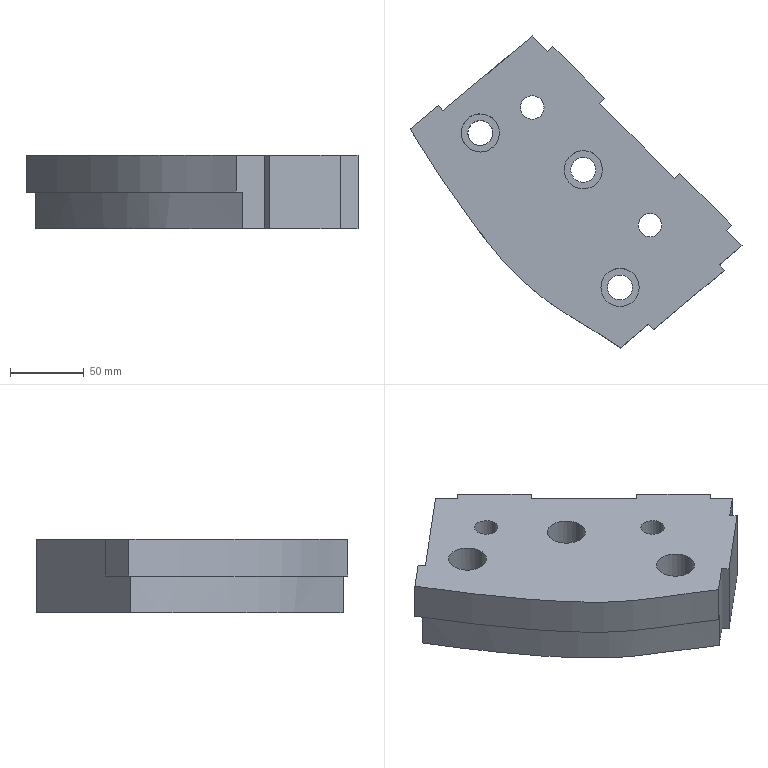Part | NX | features solid 2 | 1 solid | 33 faces | box 225.745 x 212.12 x 50 mm | volume 1112027 mm3 | plane 23 | cylinder 8 | spline 2 | commonest cylinder face diameters 17 x3 26 x3 16 x2
STEP:
#1=CARTESIAN_POINT('',(142.732,-499.403,0.));
#2=VERTEX_POINT('',#1);
#3=CARTESIAN_POINT('',(158.053,-486.547,0.));
#4=VERTEX_POINT('',#3);
#5=CARTESIAN_POINT('',(75.334,-555.957,0.));
#6=DIRECTION('',(0.766,0.6428,0.));
#7=VECTOR('',#6,1000.);
#8=LINE('',#5,#7);
#9=EDGE_CURVE('',#2,#4,#8,.T.);
#10=ORIENTED_EDGE('',*,*,#9,.F.);
#11=CARTESIAN_POINT('',(142.732,-499.403,-50.));
#12=VERTEX_POINT('',#11);
#13=CARTESIAN_POINT('',(142.732,-499.403,-50.));
#14=DIRECTION('',(0.,0.,1.));
#15=VECTOR('',#14,1000.);
#16=LINE('',#13,#15);
#17=EDGE_CURVE('',#12,#2,#16,.T.);
#18=ORIENTED_EDGE('',*,*,#17,.F.);
#19=CARTESIAN_POINT('',(158.053,-486.547,-50.));
#20=VERTEX_POINT('',#19);
#21=CARTESIAN_POINT('',(75.334,-555.957,-50.));
#22=DIRECTION('',(0.766,0.6428,0.));
#23=VECTOR('',#22,1000.);
#24=LINE('',#21,#23);
#25=EDGE_CURVE('',#12,#20,#24,.T.);
#26=ORIENTED_EDGE('',*,*,#25,.T.);
#27=CARTESIAN_POINT('',(158.053,-486.547,-50.));
#28=DIRECTION('',(0.,0.,1.));
#29=VECTOR('',#28,1000.);
#30=LINE('',#27,#29);
#31=EDGE_CURVE('',#20,#4,#30,.T.);
#32=ORIENTED_EDGE('',*,*,#31,.T.);
#33=EDGE_LOOP('',(#10,#18,#26,#32));
#34=FACE_BOUND('',#33,.T.);
#35=CARTESIAN_POINT('',(75.334,-555.957,-50.));
#36=DIRECTION('',(0.6428,-0.766,0.));
#37=DIRECTION('',(0.766,0.6428,0.));
#38=AXIS2_PLACEMENT_3D('',#35,#36,#37);
#39=PLANE('',#38);
#40=ADVANCED_FACE('',(#34),#39,.T.);
#41=CARTESIAN_POINT('',(23.477,-392.421,-50.));
#42=VERTEX_POINT('',#41);
#43=CARTESIAN_POINT('',(15.477,-392.421,-50.));
#44=DIRECTION('',(0.,0.,1.));
#45=DIRECTION('',(1.,0.,0.));
#46=AXIS2_PLACEMENT_3D('',#43,#44,#45);
#47=CIRCLE('',#46,8.);
#48=EDGE_CURVE('',#42,#42,#47,.T.);
#49=ORIENTED_EDGE('',*,*,#48,.T.);
#50=EDGE_LOOP('',(#49));
#51=FACE_BOUND('',#50,.T.);
#52=CARTESIAN_POINT('',(103.477,-472.421,-50.));
#53=VERTEX_POINT('',#52);
#54=CARTESIAN_POINT('',(95.477,-472.421,-50.));
#55=DIRECTION('',(0.,0.,1.));
#56=DIRECTION('',(1.,0.,0.));
#57=AXIS2_PLACEMENT_3D('',#54,#55,#56);
#58=CIRCLE('',#57,8.);
#59=EDGE_CURVE('',#53,#53,#58,.T.);
#60=ORIENTED_EDGE('',*,*,#59,.T.);
#61=EDGE_LOOP('',(#60));
#62=FACE_BOUND('',#61,.T.);
#63=CARTESIAN_POINT('',(61.305,-389.799,-50.));
#64=VERTEX_POINT('',#63);
#65=CARTESIAN_POINT('',(64.84,-386.263,-50.));
#66=VERTEX_POINT('',#65);
#67=CARTESIAN_POINT('',(61.305,-389.799,-50.));
#68=DIRECTION('',(0.7071,0.7071,0.));
#69=VECTOR('',#68,1000.);
#70=LINE('',#67,#69);
#71=EDGE_CURVE('',#64,#66,#70,.T.);
#72=ORIENTED_EDGE('',*,*,#71,.F.);
#73=CARTESIAN_POINT('',(112.091,-440.585,-50.));
#74=VERTEX_POINT('',#73);
#75=CARTESIAN_POINT('',(158.053,-486.547,-50.));
#76=DIRECTION('',(-0.7071,0.7071,0.));
#77=VECTOR('',#76,1000.);
#78=LINE('',#75,#77);
#79=EDGE_CURVE('',#74,#64,#78,.T.);
#80=ORIENTED_EDGE('',*,*,#79,.F.);
#81=CARTESIAN_POINT('',(115.626,-437.05,-50.));
#82=VERTEX_POINT('',#81);
#83=CARTESIAN_POINT('',(112.091,-440.585,-50.));
#84=DIRECTION('',(0.7071,0.7071,0.));
#85=VECTOR('',#84,1000.);
#86=LINE('',#83,#85);
#87=EDGE_CURVE('',#74,#82,#86,.T.);
#88=ORIENTED_EDGE('',*,*,#87,.T.);
#89=CARTESIAN_POINT('',(150.982,-472.405,-50.));
#90=VERTEX_POINT('',#89);
#91=CARTESIAN_POINT('',(161.588,-483.012,-50.));
#92=DIRECTION('',(-0.7071,0.7071,0.));
#93=VECTOR('',#92,1000.);
#94=LINE('',#91,#93);
#95=EDGE_CURVE('',#90,#82,#94,.T.);
#96=ORIENTED_EDGE('',*,*,#95,.F.);
#97=CARTESIAN_POINT('',(147.446,-475.941,-50.));
#98=VERTEX_POINT('',#97);
#99=CARTESIAN_POINT('',(147.446,-475.941,-50.));
#100=DIRECTION('',(0.7071,0.7071,0.));
#101=VECTOR('',#100,1000.);
#102=LINE('',#99,#101);
#103=EDGE_CURVE('',#98,#90,#102,.T.);
#104=ORIENTED_EDGE('',*,*,#103,.F.);
#105=CARTESIAN_POINT('',(158.053,-486.547,-50.));
#106=DIRECTION('',(-0.7071,0.7071,0.));
#107=VECTOR('',#106,1000.);
#108=LINE('',#105,#107);
#109=EDGE_CURVE('',#20,#98,#108,.T.);
#110=ORIENTED_EDGE('',*,*,#109,.F.);
#111=ORIENTED_EDGE('',*,*,#25,.F.);
#112=CARTESIAN_POINT('',(145.946,-503.233,-50.));
#113=VERTEX_POINT('',#112);
#114=CARTESIAN_POINT('',(145.946,-503.233,-50.));
#115=DIRECTION('',(-0.6428,0.766,0.));
#116=VECTOR('',#115,1000.);
#117=LINE('',#114,#116);
#118=EDGE_CURVE('',#113,#12,#117,.T.);
#119=ORIENTED_EDGE('',*,*,#118,.F.);
#120=CARTESIAN_POINT('',(97.869,-543.575,-50.));
#121=VERTEX_POINT('',#120);
#122=CARTESIAN_POINT('',(78.548,-559.787,-50.));
#123=DIRECTION('',(0.766,0.6428,0.));
#124=VECTOR('',#123,1000.);
#125=LINE('',#122,#124);
#126=EDGE_CURVE('',#121,#113,#125,.T.);
#127=ORIENTED_EDGE('',*,*,#126,.F.);
#128=CARTESIAN_POINT('',(94.655,-539.744,-50.));
#129=VERTEX_POINT('',#128);
#130=CARTESIAN_POINT('',(97.869,-543.575,-50.));
#131=DIRECTION('',(-0.6428,0.766,0.));
#132=VECTOR('',#131,1000.);
#133=LINE('',#130,#132);
#134=EDGE_CURVE('',#121,#129,#133,.T.);
#135=ORIENTED_EDGE('',*,*,#134,.T.);
#136=CARTESIAN_POINT('',(79.334,-552.6,-50.));
#137=VERTEX_POINT('',#136);
#138=CARTESIAN_POINT('',(75.334,-555.957,-50.));
#139=DIRECTION('',(0.766,0.6428,0.));
#140=VECTOR('',#139,1000.);
#141=LINE('',#138,#140);
#142=EDGE_CURVE('',#137,#129,#141,.T.);
#143=ORIENTED_EDGE('',*,*,#142,.F.);
#144=CARTESIAN_POINT('',(-61.212,-408.074,-50.));
#145=VERTEX_POINT('',#144);
#146=CARTESIAN_POINT('',(79.334,-552.6,-50.));
#147=CARTESIAN_POINT('',(78.129,-551.811,-50.));
#148=CARTESIAN_POINT('',(75.875,-550.333,-50.));
#149=CARTESIAN_POINT('',(73.445,-548.739,-50.));
#150=CARTESIAN_POINT('',(71.733,-547.614,-50.));
#151=CARTESIAN_POINT('',(70.569,-546.848,-50.));
#152=CARTESIAN_POINT('',(69.685,-546.266,-50.));
#153=CARTESIAN_POINT('',(69.138,-545.905,-50.));
#154=CARTESIAN_POINT('',(68.807,-545.687,-50.));
#155=CARTESIAN_POINT('',(68.659,-545.589,-50.));
#156=CARTESIAN_POINT('',(68.163,-545.262,-50.));
#157=CARTESIAN_POINT('',(67.633,-544.913,-50.));
#158=CARTESIAN_POINT('',(66.666,-544.277,-50.));
#159=CARTESIAN_POINT('',(65.37,-543.428,-50.));
#160=CARTESIAN_POINT('',(63.888,-542.462,-50.));
#161=CARTESIAN_POINT('',(62.033,-541.262,-50.));
#162=CARTESIAN_POINT('',(60.345,-540.182,-50.));
#163=CARTESIAN_POINT('',(59.036,-539.357,-50.));
#164=CARTESIAN_POINT('',(58.306,-538.901,-50.));
#165=CARTESIAN_POINT('',(57.852,-538.619,-50.));
#166=CARTESIAN_POINT('',(57.146,-538.183,-50.));
#167=CARTESIAN_POINT('',(56.277,-537.65,-50.));
#168=CARTESIAN_POINT('',(55.138,-536.956,-50.));
#169=CARTESIAN_POINT('',(53.756,-536.121,-50.));
#170=CARTESIAN_POINT('',(50.866,-534.395,-50.));
#171=CARTESIAN_POINT('',(47.802,-532.601,-50.));
#172=CARTESIAN_POINT('',(43.886,-530.291,-50.));
#173=CARTESIAN_POINT('',(41.125,-528.607,-50.));
#174=CARTESIAN_POINT('',(38.896,-527.213,-50.));
#175=CARTESIAN_POINT('',(37.144,-526.09,-50.));
#176=CARTESIAN_POINT('',(35.914,-525.292,-50.));
#177=CARTESIAN_POINT('',(34.476,-524.342,-50.));
#178=CARTESIAN_POINT('',(32.673,-523.128,-50.));
#179=CARTESIAN_POINT('',(30.457,-521.595,-50.));
#180=CARTESIAN_POINT('',(27.901,-519.755,-50.));
#181=CARTESIAN_POINT('',(24.674,-517.337,-50.));
#182=CARTESIAN_POINT('',(21.367,-514.704,-50.));
#183=CARTESIAN_POINT('',(18.523,-512.298,-50.));
#184=CARTESIAN_POINT('',(16.921,-510.904,-50.));
#185=CARTESIAN_POINT('',(15.67,-509.794,-50.));
#186=CARTESIAN_POINT('',(14.627,-508.851,-50.));
#187=CARTESIAN_POINT('',(13.157,-507.5,-50.));
#188=CARTESIAN_POINT('',(10.606,-505.095,-50.));
#189=CARTESIAN_POINT('',(6.904,-501.433,-50.));
#190=CARTESIAN_POINT('',(3.166,-497.511,-50.));
#191=CARTESIAN_POINT('',(0.5051,-494.599,-50.));
#192=CARTESIAN_POINT('',(-0.9962,-492.925,-50.));
#193=CARTESIAN_POINT('',(-2.202,-491.561,-50.));
#194=CARTESIAN_POINT('',(-3.122,-490.508,-50.));
#195=CARTESIAN_POINT('',(-4.455,-488.97,-50.));
#196=CARTESIAN_POINT('',(-6.754,-486.274,-50.));
#197=CARTESIAN_POINT('',(-10.105,-482.235,-50.));
#198=CARTESIAN_POINT('',(-13.491,-478.004,-50.));
#199=CARTESIAN_POINT('',(-15.906,-474.909,-50.));
#200=CARTESIAN_POINT('',(-17.269,-473.141,-50.));
#201=CARTESIAN_POINT('',(-18.366,-471.707,-50.));
#202=CARTESIAN_POINT('',(-19.197,-470.611,-50.));
#203=CARTESIAN_POINT('',(-20.41,-469.005,-50.));
#204=CARTESIAN_POINT('',(-22.512,-466.194,-50.));
#205=CARTESIAN_POINT('',(-25.61,-461.98,-50.));
#206=CARTESIAN_POINT('',(-28.785,-457.564,-50.));
#207=CARTESIAN_POINT('',(-31.069,-454.34,-50.));
#208=CARTESIAN_POINT('',(-32.371,-452.489,-50.));
#209=CARTESIAN_POINT('',(-33.403,-451.015,-50.));
#210=CARTESIAN_POINT('',(-34.256,-449.791,-50.));
#211=CARTESIAN_POINT('',(-35.453,-448.064,-50.));
#212=CARTESIAN_POINT('',(-37.515,-445.069,-50.));
#213=CARTESIAN_POINT('',(-40.462,-440.727,-50.));
#214=CARTESIAN_POINT('',(-43.972,-435.458,-50.));
#215=CARTESIAN_POINT('',(-50.953,-424.779,-50.));
#216=CARTESIAN_POINT('',(-56.683,-415.599,-50.));
#217=CARTESIAN_POINT('',(-61.212,-408.074,-50.));
#218=B_SPLINE_CURVE_WITH_KNOTS('',3,(#146,#147,#148,#149,#150,#151,#152,#153,#154,#155,#156,#157,#158,#159,#160,#161,#162,#163,#164,#165,#166,#167,#168,#169,#170,#171,#172,#173,#174,#175,#176,#177,#178,#179,#180,#181,#182,#183,#184,#185,#186,#187,#188,#189,#190,#191,#192,#193,#194,#195,#196,#197,#198,#199,#200,#201,#202,#203,#204,#205,#206,#207,#208,#209,#210,#211,#212,#213,#214,#215,#216,#217),.UNSPECIFIED.,.F.,.F.,(4,1,1,1,1,1,1,1,1,1,1,1,1,1,1,1,1,1,1,1,1,1,1,1,1,1,1,1,1,1,1,1,1,1,1,1,1,1,1,1,1,1,1,1,1,1,1,1,1,1,1,1,1,1,1,1,1,1,1,1,1,1,1,1,1,1,1,1,1,4),(0.,0.01562,0.03125,0.03906,0.04688,0.05469,0.05859,0.06055,0.0625,0.06445,0.06641,0.07031,0.07812,0.08594,0.09375,0.1094,0.1172,0.1211,0.125,0.1289,0.1328,0.1406,0.1484,0.1562,0.1875,0.2031,0.2188,0.2344,0.2422,0.25,0.2578,0.2656,0.2812,0.2969,0.3125,0.3438,0.3594,0.3672,0.375,0.3828,0.3906,0.4062,0.4375,0.4688,0.4844,0.4922,0.5,0.5078,0.5156,0.5312,0.5625,0.5938,0.6094,0.6172,0.625,0.6328,0.6406,0.6562,0.6875,0.7188,0.7344,0.7422,0.75,0.7578,0.7656,0.7812,0.8125,0.8438,0.875,1.),.UNSPECIFIED.);
#219=EDGE_CURVE('',#145,#137,#218,.F.);
#220=ORIENTED_EDGE('',*,*,#219,.F.);
#221=CARTESIAN_POINT('',(15.343,-343.837,-50.));
#222=VERTEX_POINT('',#221);
#223=CARTESIAN_POINT('',(-71.558,-416.756,-50.));
#224=DIRECTION('',(0.766,0.6428,0.));
#225=VECTOR('',#224,1000.);
#226=LINE('',#223,#225);
#227=EDGE_CURVE('',#145,#222,#226,.T.);
#228=ORIENTED_EDGE('',*,*,#227,.T.);
#229=CARTESIAN_POINT('',(25.949,-354.444,-50.));
#230=VERTEX_POINT('',#229);
#231=CARTESIAN_POINT('',(158.053,-486.547,-50.));
#232=DIRECTION('',(-0.7071,0.7071,0.));
#233=VECTOR('',#232,1000.);
#234=LINE('',#231,#233);
#235=EDGE_CURVE('',#230,#222,#234,.T.);
#236=ORIENTED_EDGE('',*,*,#235,.F.);
#237=CARTESIAN_POINT('',(29.485,-350.908,-50.));
#238=VERTEX_POINT('',#237);
#239=CARTESIAN_POINT('',(25.949,-354.444,-50.));
#240=DIRECTION('',(0.7071,0.7071,0.));
#241=VECTOR('',#240,1000.);
#242=LINE('',#239,#241);
#243=EDGE_CURVE('',#230,#238,#242,.T.);
#244=ORIENTED_EDGE('',*,*,#243,.T.);
#245=CARTESIAN_POINT('',(64.84,-386.263,-50.));
#246=DIRECTION('',(-0.7071,0.7071,0.));
#247=VECTOR('',#246,1000.);
#248=LINE('',#245,#247);
#249=EDGE_CURVE('',#66,#238,#248,.T.);
#250=ORIENTED_EDGE('',*,*,#249,.F.);
#251=EDGE_LOOP('',(#72,#80,#88,#96,#104,#110,#111,#119,#127,#135,#143,#220,#228,#236,#244,#250));
#252=FACE_BOUND('',#251,.T.);
#253=CARTESIAN_POINT('',(66.622,-514.794,-50.));
#254=VERTEX_POINT('',#253);
#255=CARTESIAN_POINT('',(75.122,-514.794,-50.));
#256=DIRECTION('',(0.,0.,-1.));
#257=DIRECTION('',(-1.,0.,0.));
#258=AXIS2_PLACEMENT_3D('',#255,#256,#257);
#259=CIRCLE('',#258,8.5);
#260=EDGE_CURVE('',#254,#254,#259,.T.);
#261=ORIENTED_EDGE('',*,*,#260,.F.);
#262=EDGE_LOOP('',(#261));
#263=FACE_BOUND('',#262,.T.);
#264=CARTESIAN_POINT('',(41.622,-434.794,-50.));
#265=VERTEX_POINT('',#264);
#266=CARTESIAN_POINT('',(50.122,-434.794,-50.));
#267=DIRECTION('',(0.,0.,-1.));
#268=DIRECTION('',(-1.,0.,0.));
#269=AXIS2_PLACEMENT_3D('',#266,#267,#268);
#270=CIRCLE('',#269,8.5);
#271=EDGE_CURVE('',#265,#265,#270,.T.);
#272=ORIENTED_EDGE('',*,*,#271,.F.);
#273=EDGE_LOOP('',(#272));
#274=FACE_BOUND('',#273,.T.);
#275=CARTESIAN_POINT('',(-28.378,-409.794,-50.));
#276=VERTEX_POINT('',#275);
#277=CARTESIAN_POINT('',(-19.878,-409.794,-50.));
#278=DIRECTION('',(0.,0.,-1.));
#279=DIRECTION('',(-1.,0.,0.));
#280=AXIS2_PLACEMENT_3D('',#277,#278,#279);
#281=CIRCLE('',#280,8.5);
#282=EDGE_CURVE('',#276,#276,#281,.T.);
#283=ORIENTED_EDGE('',*,*,#282,.F.);
#284=EDGE_LOOP('',(#283));
#285=FACE_BOUND('',#284,.T.);
#286=CARTESIAN_POINT('',(-522.658,-1199.176,-50.));
#287=DIRECTION('',(0.,0.,1.));
#288=DIRECTION('',(1.,0.,0.));
#289=AXIS2_PLACEMENT_3D('',#286,#287,#288);
#290=PLANE('',#289);
#291=ADVANCED_FACE('',(#51,#62,#252,#263,#274,#285),#290,.F.);
#292=CARTESIAN_POINT('',(23.477,-392.421,0.));
#293=VERTEX_POINT('',#292);
#294=CARTESIAN_POINT('',(15.477,-392.421,0.));
#295=DIRECTION('',(0.,0.,1.));
#296=DIRECTION('',(1.,0.,0.));
#297=AXIS2_PLACEMENT_3D('',#294,#295,#296);
#298=CIRCLE('',#297,8.);
#299=EDGE_CURVE('',#293,#293,#298,.T.);
#300=ORIENTED_EDGE('',*,*,#299,.F.);
#301=EDGE_LOOP('',(#300));
#302=FACE_BOUND('',#301,.T.);
#303=CARTESIAN_POINT('',(103.477,-472.421,0.));
#304=VERTEX_POINT('',#303);
#305=CARTESIAN_POINT('',(95.477,-472.421,0.));
#306=DIRECTION('',(0.,0.,1.));
#307=DIRECTION('',(1.,0.,0.));
#308=AXIS2_PLACEMENT_3D('',#305,#306,#307);
#309=CIRCLE('',#308,8.);
#310=EDGE_CURVE('',#304,#304,#309,.T.);
#311=ORIENTED_EDGE('',*,*,#310,.F.);
#312=EDGE_LOOP('',(#311));
#313=FACE_BOUND('',#312,.T.);
#314=CARTESIAN_POINT('',(-45.327,-394.745,0.));
#315=VERTEX_POINT('',#314);
#316=CARTESIAN_POINT('',(-48.541,-390.915,0.));
#317=VERTEX_POINT('',#316);
#318=CARTESIAN_POINT('',(-45.327,-394.745,0.));
#319=DIRECTION('',(-0.6428,0.766,0.));
#320=VECTOR('',#319,1000.);
#321=LINE('',#318,#320);
#322=EDGE_CURVE('',#315,#317,#321,.T.);
#323=ORIENTED_EDGE('',*,*,#322,.T.);
#324=CARTESIAN_POINT('',(-67.692,-406.985,0.));
#325=VERTEX_POINT('',#324);
#326=CARTESIAN_POINT('',(-67.692,-406.985,0.));
#327=DIRECTION('',(0.766,0.6428,0.));
#328=VECTOR('',#327,1000.);
#329=LINE('',#326,#328);
#330=EDGE_CURVE('',#325,#317,#329,.T.);
#331=ORIENTED_EDGE('',*,*,#330,.F.);
#332=CARTESIAN_POINT('',(75.334,-555.957,0.));
#333=VERTEX_POINT('',#332);
#334=CARTESIAN_POINT('',(-67.692,-406.985,0.));
#335=CARTESIAN_POINT('',(-63.736,-413.625,0.));
#336=CARTESIAN_POINT('',(-52.458,-432.057,0.));
#337=CARTESIAN_POINT('',(-32.602,-461.482,0.));
#338=CARTESIAN_POINT('',(-11.577,-489.134,0.));
#339=CARTESIAN_POINT('',(7.388,-509.445,0.));
#340=CARTESIAN_POINT('',(23.204,-523.049,0.));
#341=CARTESIAN_POINT('',(37.741,-532.559,0.));
#342=CARTESIAN_POINT('',(49.762,-539.511,0.));
#343=CARTESIAN_POINT('',(58.522,-544.87,0.));
#344=CARTESIAN_POINT('',(66.969,-550.477,0.));
#345=CARTESIAN_POINT('',(72.545,-554.13,0.));
#346=CARTESIAN_POINT('',(75.334,-555.957,0.));
#347=B_SPLINE_CURVE_WITH_KNOTS('',3,(#334,#335,#336,#337,#338,#339,#340,#341,#342,#343,#344,#345,#346),.UNSPECIFIED.,.F.,.F.,(4,1,1,1,1,1,1,1,1,1,4),(0.,0.1106,0.3091,0.5076,0.6069,0.7061,0.8054,0.855,0.9046,0.9523,1.),.UNSPECIFIED.);
#348=EDGE_CURVE('',#325,#333,#347,.T.);
#349=ORIENTED_EDGE('',*,*,#348,.T.);
#350=CARTESIAN_POINT('',(94.655,-539.744,0.));
#351=VERTEX_POINT('',#350);
#352=CARTESIAN_POINT('',(75.334,-555.957,0.));
#353=DIRECTION('',(0.766,0.6428,0.));
#354=VECTOR('',#353,1000.);
#355=LINE('',#352,#354);
#356=EDGE_CURVE('',#333,#351,#355,.T.);
#357=ORIENTED_EDGE('',*,*,#356,.T.);
#358=CARTESIAN_POINT('',(97.869,-543.575,0.));
#359=VERTEX_POINT('',#358);
#360=CARTESIAN_POINT('',(97.869,-543.575,0.));
#361=DIRECTION('',(-0.6428,0.766,0.));
#362=VECTOR('',#361,1000.);
#363=LINE('',#360,#362);
#364=EDGE_CURVE('',#359,#351,#363,.T.);
#365=ORIENTED_EDGE('',*,*,#364,.F.);
#366=CARTESIAN_POINT('',(145.946,-503.233,0.));
#367=VERTEX_POINT('',#366);
#368=CARTESIAN_POINT('',(78.548,-559.787,0.));
#369=DIRECTION('',(0.766,0.6428,0.));
#370=VECTOR('',#369,1000.);
#371=LINE('',#368,#370);
#372=EDGE_CURVE('',#359,#367,#371,.T.);
#373=ORIENTED_EDGE('',*,*,#372,.T.);
#374=CARTESIAN_POINT('',(145.946,-503.233,0.));
#375=DIRECTION('',(-0.6428,0.766,0.));
#376=VECTOR('',#375,1000.);
#377=LINE('',#374,#376);
#378=EDGE_CURVE('',#367,#2,#377,.T.);
#379=ORIENTED_EDGE('',*,*,#378,.T.);
#380=ORIENTED_EDGE('',*,*,#9,.T.);
#381=CARTESIAN_POINT('',(147.446,-475.941,0.));
#382=VERTEX_POINT('',#381);
#383=CARTESIAN_POINT('',(158.053,-486.547,0.));
#384=DIRECTION('',(-0.7071,0.7071,0.));
#385=VECTOR('',#384,1000.);
#386=LINE('',#383,#385);
#387=EDGE_CURVE('',#4,#382,#386,.T.);
#388=ORIENTED_EDGE('',*,*,#387,.T.);
#389=CARTESIAN_POINT('',(150.982,-472.405,0.));
#390=VERTEX_POINT('',#389);
#391=CARTESIAN_POINT('',(147.446,-475.941,0.));
#392=DIRECTION('',(0.7071,0.7071,0.));
#393=VECTOR('',#392,1000.);
#394=LINE('',#391,#393);
#395=EDGE_CURVE('',#382,#390,#394,.T.);
#396=ORIENTED_EDGE('',*,*,#395,.T.);
#397=CARTESIAN_POINT('',(115.626,-437.05,0.));
#398=VERTEX_POINT('',#397);
#399=CARTESIAN_POINT('',(161.588,-483.012,0.));
#400=DIRECTION('',(-0.7071,0.7071,0.));
#401=VECTOR('',#400,1000.);
#402=LINE('',#399,#401);
#403=EDGE_CURVE('',#390,#398,#402,.T.);
#404=ORIENTED_EDGE('',*,*,#403,.T.);
#405=CARTESIAN_POINT('',(112.091,-440.585,0.));
#406=VERTEX_POINT('',#405);
#407=CARTESIAN_POINT('',(112.091,-440.585,0.));
#408=DIRECTION('',(0.7071,0.7071,0.));
#409=VECTOR('',#408,1000.);
#410=LINE('',#407,#409);
#411=EDGE_CURVE('',#406,#398,#410,.T.);
#412=ORIENTED_EDGE('',*,*,#411,.F.);
#413=CARTESIAN_POINT('',(61.305,-389.799,0.));
#414=VERTEX_POINT('',#413);
#415=CARTESIAN_POINT('',(158.053,-486.547,0.));
#416=DIRECTION('',(-0.7071,0.7071,0.));
#417=VECTOR('',#416,1000.);
#418=LINE('',#415,#417);
#419=EDGE_CURVE('',#406,#414,#418,.T.);
#420=ORIENTED_EDGE('',*,*,#419,.T.);
#421=CARTESIAN_POINT('',(64.84,-386.263,0.));
#422=VERTEX_POINT('',#421);
#423=CARTESIAN_POINT('',(61.305,-389.799,0.));
#424=DIRECTION('',(0.7071,0.7071,0.));
#425=VECTOR('',#424,1000.);
#426=LINE('',#423,#425);
#427=EDGE_CURVE('',#414,#422,#426,.T.);
#428=ORIENTED_EDGE('',*,*,#427,.T.);
#429=CARTESIAN_POINT('',(29.485,-350.908,0.));
#430=VERTEX_POINT('',#429);
#431=CARTESIAN_POINT('',(64.84,-386.263,0.));
#432=DIRECTION('',(-0.7071,0.7071,0.));
#433=VECTOR('',#432,1000.);
#434=LINE('',#431,#433);
#435=EDGE_CURVE('',#422,#430,#434,.T.);
#436=ORIENTED_EDGE('',*,*,#435,.T.);
#437=CARTESIAN_POINT('',(25.949,-354.444,0.));
#438=VERTEX_POINT('',#437);
#439=CARTESIAN_POINT('',(25.949,-354.444,0.));
#440=DIRECTION('',(0.7071,0.7071,0.));
#441=VECTOR('',#440,1000.);
#442=LINE('',#439,#441);
#443=EDGE_CURVE('',#438,#430,#442,.T.);
#444=ORIENTED_EDGE('',*,*,#443,.F.);
#445=CARTESIAN_POINT('',(15.343,-343.837,0.));
#446=VERTEX_POINT('',#445);
#447=CARTESIAN_POINT('',(158.053,-486.547,0.));
#448=DIRECTION('',(-0.7071,0.7071,0.));
#449=VECTOR('',#448,1000.);
#450=LINE('',#447,#449);
#451=EDGE_CURVE('',#438,#446,#450,.T.);
#452=ORIENTED_EDGE('',*,*,#451,.T.);
#453=CARTESIAN_POINT('',(-64.478,-410.815,0.));
#454=DIRECTION('',(0.766,0.6428,0.));
#455=VECTOR('',#454,1000.);
#456=LINE('',#453,#455);
#457=EDGE_CURVE('',#315,#446,#456,.T.);
#458=ORIENTED_EDGE('',*,*,#457,.F.);
#459=EDGE_LOOP('',(#323,#331,#349,#357,#365,#373,#379,#380,#388,#396,#404,#412,#420,#428,#436,#444,#452,#458));
#460=FACE_BOUND('',#459,.T.);
#461=CARTESIAN_POINT('',(62.122,-514.794,0.));
#462=VERTEX_POINT('',#461);
#463=CARTESIAN_POINT('',(75.122,-514.794,0.));
#464=DIRECTION('',(0.,0.,-1.));
#465=DIRECTION('',(-1.,0.,0.));
#466=AXIS2_PLACEMENT_3D('',#463,#464,#465);
#467=CIRCLE('',#466,13.);
#468=EDGE_CURVE('',#462,#462,#467,.T.);
#469=ORIENTED_EDGE('',*,*,#468,.T.);
#470=EDGE_LOOP('',(#469));
#471=FACE_BOUND('',#470,.T.);
#472=CARTESIAN_POINT('',(63.122,-434.794,0.));
#473=VERTEX_POINT('',#472);
#474=CARTESIAN_POINT('',(50.122,-434.794,0.));
#475=DIRECTION('',(0.,0.,1.));
#476=DIRECTION('',(1.,0.,0.));
#477=AXIS2_PLACEMENT_3D('',#474,#475,#476);
#478=CIRCLE('',#477,13.);
#479=EDGE_CURVE('',#473,#473,#478,.T.);
#480=ORIENTED_EDGE('',*,*,#479,.F.);
#481=EDGE_LOOP('',(#480));
#482=FACE_BOUND('',#481,.T.);
#483=CARTESIAN_POINT('',(-32.878,-409.794,0.));
#484=VERTEX_POINT('',#483);
#485=CARTESIAN_POINT('',(-19.878,-409.794,0.));
#486=DIRECTION('',(0.,0.,-1.));
#487=DIRECTION('',(-1.,0.,0.));
#488=AXIS2_PLACEMENT_3D('',#485,#486,#487);
#489=CIRCLE('',#488,13.);
#490=EDGE_CURVE('',#484,#484,#489,.T.);
#491=ORIENTED_EDGE('',*,*,#490,.T.);
#492=EDGE_LOOP('',(#491));
#493=FACE_BOUND('',#492,.T.);
#494=CARTESIAN_POINT('',(-522.658,-1199.176,0.));
#495=DIRECTION('',(0.,0.,1.));
#496=DIRECTION('',(1.,0.,0.));
#497=AXIS2_PLACEMENT_3D('',#494,#495,#496);
#498=PLANE('',#497);
#499=ADVANCED_FACE('',(#302,#313,#460,#471,#482,#493),#498,.T.);
#500=CARTESIAN_POINT('',(-19.878,-401.294,-25.));
#501=VERTEX_POINT('',#500);
#502=CARTESIAN_POINT('',(-19.878,-409.794,-25.));
#503=DIRECTION('',(0.,0.,-1.));
#504=DIRECTION('',(0.,1.,0.));
#505=AXIS2_PLACEMENT_3D('',#502,#503,#504);
#506=CIRCLE('',#505,8.5);
#507=EDGE_CURVE('',#501,#501,#506,.F.);
#508=ORIENTED_EDGE('',*,*,#507,.T.);
#509=EDGE_LOOP('',(#508));
#510=FACE_BOUND('',#509,.T.);
#511=ORIENTED_EDGE('',*,*,#282,.T.);
#512=EDGE_LOOP('',(#511));
#513=FACE_BOUND('',#512,.T.);
#514=CARTESIAN_POINT('',(-19.878,-409.794,-75.));
#515=DIRECTION('',(0.,0.,1.));
#516=DIRECTION('',(0.,-1.,0.));
#517=AXIS2_PLACEMENT_3D('',#514,#515,#516);
#518=CYLINDRICAL_SURFACE('',#517,8.5);
#519=ADVANCED_FACE('',(#510,#513),#518,.F.);
#520=ORIENTED_EDGE('',*,*,#507,.F.);
#521=EDGE_LOOP('',(#520));
#522=FACE_BOUND('',#521,.T.);
#523=CARTESIAN_POINT('',(-19.878,-422.794,-25.));
#524=VERTEX_POINT('',#523);
#525=CARTESIAN_POINT('',(-19.878,-409.794,-25.));
#526=DIRECTION('',(0.,0.,1.));
#527=DIRECTION('',(0.,-1.,0.));
#528=AXIS2_PLACEMENT_3D('',#525,#526,#527);
#529=CIRCLE('',#528,13.);
#530=EDGE_CURVE('',#524,#524,#529,.T.);
#531=ORIENTED_EDGE('',*,*,#530,.T.);
#532=EDGE_LOOP('',(#531));
#533=FACE_BOUND('',#532,.T.);
#534=CARTESIAN_POINT('',(-19.878,-409.794,-25.));
#535=DIRECTION('',(0.,0.,-1.));
#536=DIRECTION('',(0.,1.,0.));
#537=AXIS2_PLACEMENT_3D('',#534,#535,#536);
#538=PLANE('',#537);
#539=ADVANCED_FACE('',(#522,#533),#538,.F.);
#540=ORIENTED_EDGE('',*,*,#530,.F.);
#541=EDGE_LOOP('',(#540));
#542=FACE_BOUND('',#541,.T.);
#543=ORIENTED_EDGE('',*,*,#490,.F.);
#544=EDGE_LOOP('',(#543));
#545=FACE_BOUND('',#544,.T.);
#546=CARTESIAN_POINT('',(-19.878,-409.794,-25.));
#547=DIRECTION('',(0.,0.,1.));
#548=DIRECTION('',(0.,-1.,0.));
#549=AXIS2_PLACEMENT_3D('',#546,#547,#548);
#550=CYLINDRICAL_SURFACE('',#549,13.);
#551=ADVANCED_FACE('',(#542,#545),#550,.F.);
#552=CARTESIAN_POINT('',(94.655,-539.744,-42.5));
#553=DIRECTION('',(0.,0.,1.));
#554=VECTOR('',#553,1000.);
#555=LINE('',#552,#554);
#556=EDGE_CURVE('',#129,#351,#555,.T.);
#557=ORIENTED_EDGE('',*,*,#556,.T.);
#558=ORIENTED_EDGE('',*,*,#356,.F.);
#559=CARTESIAN_POINT('',(75.334,-555.957,-25.));
#560=VERTEX_POINT('',#559);
#561=CARTESIAN_POINT('',(75.334,-555.957,-50.));
#562=DIRECTION('',(0.,0.,1.));
#563=VECTOR('',#562,1000.);
#564=LINE('',#561,#563);
#565=EDGE_CURVE('',#560,#333,#564,.T.);
#566=ORIENTED_EDGE('',*,*,#565,.F.);
#567=CARTESIAN_POINT('',(79.334,-552.6,-25.));
#568=VERTEX_POINT('',#567);
#569=CARTESIAN_POINT('',(75.334,-555.957,-25.));
#570=DIRECTION('',(-0.766,-0.6428,0.));
#571=VECTOR('',#570,1000.);
#572=LINE('',#569,#571);
#573=EDGE_CURVE('',#568,#560,#572,.T.);
#574=ORIENTED_EDGE('',*,*,#573,.F.);
#575=CARTESIAN_POINT('',(79.334,-552.6,-42.5));
#576=DIRECTION('',(0.,0.,-1.));
#577=VECTOR('',#576,1000.);
#578=LINE('',#575,#577);
#579=EDGE_CURVE('',#137,#568,#578,.F.);
#580=ORIENTED_EDGE('',*,*,#579,.F.);
#581=ORIENTED_EDGE('',*,*,#142,.T.);
#582=EDGE_LOOP('',(#557,#558,#566,#574,#580,#581));
#583=FACE_BOUND('',#582,.T.);
#584=CARTESIAN_POINT('',(75.334,-555.957,-50.));
#585=DIRECTION('',(0.6428,-0.766,0.));
#586=DIRECTION('',(0.766,0.6428,0.));
#587=AXIS2_PLACEMENT_3D('',#584,#585,#586);
#588=PLANE('',#587);
#589=ADVANCED_FACE('',(#583),#588,.T.);
#590=ORIENTED_EDGE('',*,*,#95,.T.);
#591=CARTESIAN_POINT('',(115.626,-437.05,-50.));
#592=DIRECTION('',(0.,0.,1.));
#593=VECTOR('',#592,1000.);
#594=LINE('',#591,#593);
#595=EDGE_CURVE('',#82,#398,#594,.T.);
#596=ORIENTED_EDGE('',*,*,#595,.T.);
#597=ORIENTED_EDGE('',*,*,#403,.F.);
#598=CARTESIAN_POINT('',(150.982,-472.405,-50.));
#599=DIRECTION('',(0.,0.,1.));
#600=VECTOR('',#599,1000.);
#601=LINE('',#598,#600);
#602=EDGE_CURVE('',#90,#390,#601,.T.);
#603=ORIENTED_EDGE('',*,*,#602,.F.);
#604=EDGE_LOOP('',(#590,#596,#597,#603));
#605=FACE_BOUND('',#604,.T.);
#606=CARTESIAN_POINT('',(161.588,-483.012,-50.));
#607=DIRECTION('',(0.7071,0.7071,0.));
#608=DIRECTION('',(-0.7071,0.7071,0.));
#609=AXIS2_PLACEMENT_3D('',#606,#607,#608);
#610=PLANE('',#609);
#611=ADVANCED_FACE('',(#605),#610,.T.);
#612=ORIENTED_EDGE('',*,*,#602,.T.);
#613=ORIENTED_EDGE('',*,*,#395,.F.);
#614=CARTESIAN_POINT('',(147.446,-475.941,-50.));
#615=DIRECTION('',(0.,0.,1.));
#616=VECTOR('',#615,1000.);
#617=LINE('',#614,#616);
#618=EDGE_CURVE('',#98,#382,#617,.T.);
#619=ORIENTED_EDGE('',*,*,#618,.F.);
#620=ORIENTED_EDGE('',*,*,#103,.T.);
#621=EDGE_LOOP('',(#612,#613,#619,#620));
#622=FACE_BOUND('',#621,.T.);
#623=CARTESIAN_POINT('',(147.446,-475.941,-50.));
#624=DIRECTION('',(-0.7071,0.7071,0.));
#625=DIRECTION('',(-0.7071,-0.7071,0.));
#626=AXIS2_PLACEMENT_3D('',#623,#624,#625);
#627=PLANE('',#626);
#628=ADVANCED_FACE('',(#622),#627,.F.);
#629=ORIENTED_EDGE('',*,*,#109,.T.);
#630=ORIENTED_EDGE('',*,*,#618,.T.);
#631=ORIENTED_EDGE('',*,*,#387,.F.);
#632=ORIENTED_EDGE('',*,*,#31,.F.);
#633=EDGE_LOOP('',(#629,#630,#631,#632));
#634=FACE_BOUND('',#633,.T.);
#635=CARTESIAN_POINT('',(158.053,-486.547,-50.));
#636=DIRECTION('',(0.7071,0.7071,0.));
#637=DIRECTION('',(-0.7071,0.7071,0.));
#638=AXIS2_PLACEMENT_3D('',#635,#636,#637);
#639=PLANE('',#638);
#640=ADVANCED_FACE('',(#634),#639,.T.);
#641=CARTESIAN_POINT('',(88.122,-514.794,-25.));
#642=VERTEX_POINT('',#641);
#643=CARTESIAN_POINT('',(75.122,-514.794,-25.));
#644=DIRECTION('',(0.,0.,1.));
#645=DIRECTION('',(1.,0.,0.));
#646=AXIS2_PLACEMENT_3D('',#643,#644,#645);
#647=CIRCLE('',#646,13.);
#648=EDGE_CURVE('',#642,#642,#647,.T.);
#649=ORIENTED_EDGE('',*,*,#648,.F.);
#650=EDGE_LOOP('',(#649));
#651=FACE_BOUND('',#650,.T.);
#652=ORIENTED_EDGE('',*,*,#468,.F.);
#653=EDGE_LOOP('',(#652));
#654=FACE_BOUND('',#653,.T.);
#655=CARTESIAN_POINT('',(75.122,-514.794,-25.));
#656=DIRECTION('',(0.,0.,1.));
#657=DIRECTION('',(1.,0.,0.));
#658=AXIS2_PLACEMENT_3D('',#655,#656,#657);
#659=CYLINDRICAL_SURFACE('',#658,13.);
#660=ADVANCED_FACE('',(#651,#654),#659,.F.);
#661=CARTESIAN_POINT('',(66.622,-514.794,-25.));
#662=VERTEX_POINT('',#661);
#663=CARTESIAN_POINT('',(75.122,-514.794,-25.));
#664=DIRECTION('',(0.,0.,-1.));
#665=DIRECTION('',(-1.,0.,0.));
#666=AXIS2_PLACEMENT_3D('',#663,#664,#665);
#667=CIRCLE('',#666,8.5);
#668=EDGE_CURVE('',#662,#662,#667,.F.);
#669=ORIENTED_EDGE('',*,*,#668,.F.);
#670=EDGE_LOOP('',(#669));
#671=FACE_BOUND('',#670,.T.);
#672=ORIENTED_EDGE('',*,*,#648,.T.);
#673=EDGE_LOOP('',(#672));
#674=FACE_BOUND('',#673,.T.);
#675=CARTESIAN_POINT('',(75.122,-514.794,-25.));
#676=DIRECTION('',(0.,0.,-1.));
#677=DIRECTION('',(-1.,0.,0.));
#678=AXIS2_PLACEMENT_3D('',#675,#676,#677);
#679=PLANE('',#678);
#680=ADVANCED_FACE('',(#671,#674),#679,.F.);
#681=ORIENTED_EDGE('',*,*,#260,.T.);
#682=EDGE_LOOP('',(#681));
#683=FACE_BOUND('',#682,.T.);
#684=ORIENTED_EDGE('',*,*,#668,.T.);
#685=EDGE_LOOP('',(#684));
#686=FACE_BOUND('',#685,.T.);
#687=CARTESIAN_POINT('',(75.122,-514.794,-75.));
#688=DIRECTION('',(0.,0.,1.));
#689=DIRECTION('',(1.,0.,0.));
#690=AXIS2_PLACEMENT_3D('',#687,#688,#689);
#691=CYLINDRICAL_SURFACE('',#690,8.5);
#692=ADVANCED_FACE('',(#683,#686),#691,.F.);
#693=ORIENTED_EDGE('',*,*,#411,.T.);
#694=ORIENTED_EDGE('',*,*,#595,.F.);
#695=ORIENTED_EDGE('',*,*,#87,.F.);
#696=CARTESIAN_POINT('',(112.091,-440.585,-50.));
#697=DIRECTION('',(0.,0.,1.));
#698=VECTOR('',#697,1000.);
#699=LINE('',#696,#698);
#700=EDGE_CURVE('',#74,#406,#699,.T.);
#701=ORIENTED_EDGE('',*,*,#700,.T.);
#702=EDGE_LOOP('',(#693,#694,#695,#701));
#703=FACE_BOUND('',#702,.T.);
#704=CARTESIAN_POINT('',(112.091,-440.585,-50.));
#705=DIRECTION('',(-0.7071,0.7071,0.));
#706=DIRECTION('',(-0.7071,-0.7071,0.));
#707=AXIS2_PLACEMENT_3D('',#704,#705,#706);
#708=PLANE('',#707);
#709=ADVANCED_FACE('',(#703),#708,.T.);
#710=ORIENTED_EDGE('',*,*,#79,.T.);
#711=CARTESIAN_POINT('',(61.305,-389.799,-50.));
#712=DIRECTION('',(0.,0.,1.));
#713=VECTOR('',#712,1000.);
#714=LINE('',#711,#713);
#715=EDGE_CURVE('',#64,#414,#714,.T.);
#716=ORIENTED_EDGE('',*,*,#715,.T.);
#717=ORIENTED_EDGE('',*,*,#419,.F.);
#718=ORIENTED_EDGE('',*,*,#700,.F.);
#719=EDGE_LOOP('',(#710,#716,#717,#718));
#720=FACE_BOUND('',#719,.T.);
#721=CARTESIAN_POINT('',(158.053,-486.547,-50.));
#722=DIRECTION('',(0.7071,0.7071,0.));
#723=DIRECTION('',(-0.7071,0.7071,0.));
#724=AXIS2_PLACEMENT_3D('',#721,#722,#723);
#725=PLANE('',#724);
#726=ADVANCED_FACE('',(#720),#725,.T.);
#727=CARTESIAN_POINT('',(63.122,-434.794,-25.));
#728=VERTEX_POINT('',#727);
#729=CARTESIAN_POINT('',(50.122,-434.794,-25.));
#730=DIRECTION('',(0.,0.,1.));
#731=DIRECTION('',(1.,0.,0.));
#732=AXIS2_PLACEMENT_3D('',#729,#730,#731);
#733=CIRCLE('',#732,13.);
#734=EDGE_CURVE('',#728,#728,#733,.T.);
#735=ORIENTED_EDGE('',*,*,#734,.F.);
#736=EDGE_LOOP('',(#735));
#737=FACE_BOUND('',#736,.T.);
#738=ORIENTED_EDGE('',*,*,#479,.T.);
#739=EDGE_LOOP('',(#738));
#740=FACE_BOUND('',#739,.T.);
#741=CARTESIAN_POINT('',(50.122,-434.794,-25.));
#742=DIRECTION('',(0.,0.,1.));
#743=DIRECTION('',(1.,0.,0.));
#744=AXIS2_PLACEMENT_3D('',#741,#742,#743);
#745=CYLINDRICAL_SURFACE('',#744,13.);
#746=ADVANCED_FACE('',(#737,#740),#745,.F.);
#747=ORIENTED_EDGE('',*,*,#271,.T.);
#748=EDGE_LOOP('',(#747));
#749=FACE_BOUND('',#748,.T.);
#750=CARTESIAN_POINT('',(41.622,-434.794,-25.));
#751=VERTEX_POINT('',#750);
#752=CARTESIAN_POINT('',(50.122,-434.794,-25.));
#753=DIRECTION('',(0.,0.,-1.));
#754=DIRECTION('',(-1.,0.,0.));
#755=AXIS2_PLACEMENT_3D('',#752,#753,#754);
#756=CIRCLE('',#755,8.5);
#757=EDGE_CURVE('',#751,#751,#756,.F.);
#758=ORIENTED_EDGE('',*,*,#757,.T.);
#759=EDGE_LOOP('',(#758));
#760=FACE_BOUND('',#759,.T.);
#761=CARTESIAN_POINT('',(50.122,-434.794,-75.));
#762=DIRECTION('',(0.,0.,1.));
#763=DIRECTION('',(1.,0.,0.));
#764=AXIS2_PLACEMENT_3D('',#761,#762,#763);
#765=CYLINDRICAL_SURFACE('',#764,8.5);
#766=ADVANCED_FACE('',(#749,#760),#765,.F.);
#767=ORIENTED_EDGE('',*,*,#757,.F.);
#768=EDGE_LOOP('',(#767));
#769=FACE_BOUND('',#768,.T.);
#770=ORIENTED_EDGE('',*,*,#734,.T.);
#771=EDGE_LOOP('',(#770));
#772=FACE_BOUND('',#771,.T.);
#773=CARTESIAN_POINT('',(50.122,-434.794,-25.));
#774=DIRECTION('',(0.,0.,-1.));
#775=DIRECTION('',(-1.,0.,0.));
#776=AXIS2_PLACEMENT_3D('',#773,#774,#775);
#777=PLANE('',#776);
#778=ADVANCED_FACE('',(#769,#772),#777,.F.);
#779=CARTESIAN_POINT('',(-61.212,-408.074,-25.));
#780=VERTEX_POINT('',#779);
#781=CARTESIAN_POINT('',(-61.212,-408.074,-37.5));
#782=DIRECTION('',(0.,0.,-1.));
#783=VECTOR('',#782,1000.);
#784=LINE('',#781,#783);
#785=EDGE_CURVE('',#145,#780,#784,.F.);
#786=ORIENTED_EDGE('',*,*,#785,.F.);
#787=ORIENTED_EDGE('',*,*,#219,.T.);
#788=ORIENTED_EDGE('',*,*,#579,.T.);
#789=CARTESIAN_POINT('',(-61.212,-408.074,-25.));
#790=CARTESIAN_POINT('',(-56.79,-415.423,-25.));
#791=CARTESIAN_POINT('',(-47.746,-429.971,-25.));
#792=CARTESIAN_POINT('',(-33.386,-451.282,-25.));
#793=CARTESIAN_POINT('',(-18.335,-472.118,-25.));
#794=CARTESIAN_POINT('',(-2.306,-492.005,-25.));
#795=CARTESIAN_POINT('',(12.335,-507.213,-25.));
#796=CARTESIAN_POINT('',(25.194,-517.921,-25.));
#797=CARTESIAN_POINT('',(35.465,-525.162,-25.));
#798=CARTESIAN_POINT('',(46.254,-531.741,-25.));
#799=CARTESIAN_POINT('',(57.594,-538.315,-25.));
#800=CARTESIAN_POINT('',(68.58,-545.537,-25.));
#801=CARTESIAN_POINT('',(75.727,-550.237,-25.));
#802=CARTESIAN_POINT('',(79.334,-552.6,-25.));
#803=B_SPLINE_CURVE_WITH_KNOTS('',3,(#789,#790,#791,#792,#793,#794,#795,#796,#797,#798,#799,#800,#801,#802),.UNSPECIFIED.,.F.,.F.,(4,1,1,1,1,1,1,1,1,1,1,4),(0.02038,0.1437,0.2671,0.3904,0.5138,0.6371,0.6988,0.7605,0.8222,0.8838,0.9455,1.007),.UNSPECIFIED.);
#804=EDGE_CURVE('',#780,#568,#803,.T.);
#805=ORIENTED_EDGE('',*,*,#804,.F.);
#806=EDGE_LOOP('',(#786,#787,#788,#805));
#807=FACE_BOUND('',#806,.T.);
#808=CARTESIAN_POINT('',(-61.212,-408.074,-25.));
#809=CARTESIAN_POINT('',(-61.212,-408.074,-50.));
#810=CARTESIAN_POINT('',(-56.79,-415.423,-25.));
#811=CARTESIAN_POINT('',(-56.79,-415.423,-50.));
#812=CARTESIAN_POINT('',(-47.746,-429.971,-25.));
#813=CARTESIAN_POINT('',(-47.746,-429.971,-50.));
#814=CARTESIAN_POINT('',(-33.386,-451.282,-25.));
#815=CARTESIAN_POINT('',(-33.386,-451.282,-50.));
#816=CARTESIAN_POINT('',(-18.335,-472.118,-25.));
#817=CARTESIAN_POINT('',(-18.335,-472.118,-50.));
#818=CARTESIAN_POINT('',(-2.306,-492.005,-25.));
#819=CARTESIAN_POINT('',(-2.306,-492.005,-50.));
#820=CARTESIAN_POINT('',(12.335,-507.213,-25.));
#821=CARTESIAN_POINT('',(12.335,-507.213,-50.));
#822=CARTESIAN_POINT('',(25.194,-517.921,-25.));
#823=CARTESIAN_POINT('',(25.194,-517.921,-50.));
#824=CARTESIAN_POINT('',(35.465,-525.162,-25.));
#825=CARTESIAN_POINT('',(35.465,-525.162,-50.));
#826=CARTESIAN_POINT('',(46.254,-531.741,-25.));
#827=CARTESIAN_POINT('',(46.254,-531.741,-50.));
#828=CARTESIAN_POINT('',(57.594,-538.315,-25.));
#829=CARTESIAN_POINT('',(57.594,-538.315,-50.));
#830=CARTESIAN_POINT('',(68.58,-545.537,-25.));
#831=CARTESIAN_POINT('',(68.58,-545.537,-50.));
#832=CARTESIAN_POINT('',(75.727,-550.237,-25.));
#833=CARTESIAN_POINT('',(75.727,-550.237,-50.));
#834=CARTESIAN_POINT('',(79.334,-552.6,-25.));
#835=CARTESIAN_POINT('',(79.334,-552.6,-50.));
#836=B_SPLINE_SURFACE_WITH_KNOTS('',3,1,((#808,#809),(#810,#811),(#812,#813),(#814,#815),(#816,#817),(#818,#819),(#820,#821),(#822,#823),(#824,#825),(#826,#827),(#828,#829),(#830,#831),(#832,#833),(#834,#835)),.SURF_OF_LINEAR_EXTRUSION.,.F.,.F.,.F.,(4,1,1,1,1,1,1,1,1,1,1,4),(2,2),(0.02038,0.1437,0.2671,0.3904,0.5138,0.6371,0.6988,0.7605,0.8222,0.8838,0.9455,1.007),(0.,1.),.UNSPECIFIED.);
#837=ADVANCED_FACE('',(#807),#836,.F.);
#838=CARTESIAN_POINT('',(-67.692,-406.985,-25.));
#839=VERTEX_POINT('',#838);
#840=CARTESIAN_POINT('',(-67.692,-406.985,-25.));
#841=CARTESIAN_POINT('',(-63.736,-413.625,-25.));
#842=CARTESIAN_POINT('',(-52.458,-432.057,-25.));
#843=CARTESIAN_POINT('',(-32.602,-461.482,-25.));
#844=CARTESIAN_POINT('',(-11.577,-489.134,-25.));
#845=CARTESIAN_POINT('',(7.388,-509.445,-25.));
#846=CARTESIAN_POINT('',(23.204,-523.049,-25.));
#847=CARTESIAN_POINT('',(37.741,-532.559,-25.));
#848=CARTESIAN_POINT('',(49.762,-539.511,-25.));
#849=CARTESIAN_POINT('',(58.522,-544.87,-25.));
#850=CARTESIAN_POINT('',(66.969,-550.477,-25.));
#851=CARTESIAN_POINT('',(72.545,-554.13,-25.));
#852=CARTESIAN_POINT('',(75.334,-555.957,-25.));
#853=B_SPLINE_CURVE_WITH_KNOTS('',3,(#840,#841,#842,#843,#844,#845,#846,#847,#848,#849,#850,#851,#852),.UNSPECIFIED.,.F.,.F.,(4,1,1,1,1,1,1,1,1,1,4),(0.,0.1106,0.3091,0.5076,0.6069,0.7061,0.8054,0.855,0.9046,0.9523,1.),.UNSPECIFIED.);
#854=EDGE_CURVE('',#560,#839,#853,.F.);
#855=ORIENTED_EDGE('',*,*,#854,.F.);
#856=ORIENTED_EDGE('',*,*,#565,.T.);
#857=ORIENTED_EDGE('',*,*,#348,.F.);
#858=CARTESIAN_POINT('',(-67.692,-406.985,-50.));
#859=DIRECTION('',(0.,0.,1.));
#860=VECTOR('',#859,1000.);
#861=LINE('',#858,#860);
#862=EDGE_CURVE('',#839,#325,#861,.T.);
#863=ORIENTED_EDGE('',*,*,#862,.F.);
#864=EDGE_LOOP('',(#855,#856,#857,#863));
#865=FACE_BOUND('',#864,.T.);
#866=CARTESIAN_POINT('',(-67.692,-406.985,-25.));
#867=CARTESIAN_POINT('',(-67.692,-406.985,0.));
#868=CARTESIAN_POINT('',(-63.22,-414.492,-25.));
#869=CARTESIAN_POINT('',(-63.22,-414.492,0.));
#870=CARTESIAN_POINT('',(-54.073,-429.388,-25.));
#871=CARTESIAN_POINT('',(-54.073,-429.388,0.));
#872=CARTESIAN_POINT('',(-39.535,-451.203,-25.));
#873=CARTESIAN_POINT('',(-39.535,-451.203,0.));
#874=CARTESIAN_POINT('',(-24.275,-472.545,-25.));
#875=CARTESIAN_POINT('',(-24.275,-472.545,0.));
#876=CARTESIAN_POINT('',(-7.98,-493.083,-25.));
#877=CARTESIAN_POINT('',(-7.98,-493.083,0.));
#878=CARTESIAN_POINT('',(9.98,-512.262,-25.));
#879=CARTESIAN_POINT('',(9.98,-512.262,0.));
#880=CARTESIAN_POINT('',(27.168,-525.837,-25.));
#881=CARTESIAN_POINT('',(27.168,-525.837,0.));
#882=CARTESIAN_POINT('',(42.022,-535.075,-25.));
#883=CARTESIAN_POINT('',(42.022,-535.075,0.));
#884=CARTESIAN_POINT('',(57.175,-543.797,-25.));
#885=CARTESIAN_POINT('',(57.175,-543.797,0.));
#886=CARTESIAN_POINT('',(68.023,-551.168,-25.));
#887=CARTESIAN_POINT('',(68.023,-551.168,0.));
#888=CARTESIAN_POINT('',(75.334,-555.957,-25.));
#889=CARTESIAN_POINT('',(75.334,-555.957,0.));
#890=B_SPLINE_SURFACE_WITH_KNOTS('',3,1,((#866,#867),(#868,#869),(#870,#871),(#872,#873),(#874,#875),(#876,#877),(#878,#879),(#880,#881),(#882,#883),(#884,#885),(#886,#887),(#888,#889)),.SURF_OF_LINEAR_EXTRUSION.,.F.,.F.,.F.,(4,1,1,1,1,1,1,1,1,4),(2,2),(0.,0.125,0.25,0.375,0.5,0.625,0.75,0.8125,0.875,1.),(0.,1.),.UNSPECIFIED.);
#891=ADVANCED_FACE('',(#865),#890,.T.);
#892=ORIENTED_EDGE('',*,*,#330,.T.);
#893=CARTESIAN_POINT('',(-48.541,-390.915,-25.));
#894=VERTEX_POINT('',#893);
#895=CARTESIAN_POINT('',(-48.541,-390.915,-50.));
#896=DIRECTION('',(0.,0.,-1.));
#897=VECTOR('',#896,1000.);
#898=LINE('',#895,#897);
#899=EDGE_CURVE('',#317,#894,#898,.T.);
#900=ORIENTED_EDGE('',*,*,#899,.T.);
#901=CARTESIAN_POINT('',(-67.692,-406.985,-25.));
#902=DIRECTION('',(-0.766,-0.6428,0.));
#903=VECTOR('',#902,1000.);
#904=LINE('',#901,#903);
#905=EDGE_CURVE('',#894,#839,#904,.T.);
#906=ORIENTED_EDGE('',*,*,#905,.T.);
#907=ORIENTED_EDGE('',*,*,#862,.T.);
#908=EDGE_LOOP('',(#892,#900,#906,#907));
#909=FACE_BOUND('',#908,.T.);
#910=CARTESIAN_POINT('',(-67.692,-406.985,-50.));
#911=DIRECTION('',(0.6428,-0.766,0.));
#912=DIRECTION('',(0.766,0.6428,0.));
#913=AXIS2_PLACEMENT_3D('',#910,#911,#912);
#914=PLANE('',#913);
#915=ADVANCED_FACE('',(#909),#914,.F.);
#916=CARTESIAN_POINT('',(15.343,-343.837,-50.));
#917=DIRECTION('',(0.,0.,1.));
#918=VECTOR('',#917,1000.);
#919=LINE('',#916,#918);
#920=EDGE_CURVE('',#222,#446,#919,.T.);
#921=ORIENTED_EDGE('',*,*,#920,.T.);
#922=ORIENTED_EDGE('',*,*,#451,.F.);
#923=CARTESIAN_POINT('',(25.949,-354.444,-50.));
#924=DIRECTION('',(0.,0.,1.));
#925=VECTOR('',#924,1000.);
#926=LINE('',#923,#925);
#927=EDGE_CURVE('',#230,#438,#926,.T.);
#928=ORIENTED_EDGE('',*,*,#927,.F.);
#929=ORIENTED_EDGE('',*,*,#235,.T.);
#930=EDGE_LOOP('',(#921,#922,#928,#929));
#931=FACE_BOUND('',#930,.T.);
#932=CARTESIAN_POINT('',(158.053,-486.547,-50.));
#933=DIRECTION('',(0.7071,0.7071,0.));
#934=DIRECTION('',(-0.7071,0.7071,0.));
#935=AXIS2_PLACEMENT_3D('',#932,#933,#934);
#936=PLANE('',#935);
#937=ADVANCED_FACE('',(#931),#936,.T.);
#938=CARTESIAN_POINT('',(29.485,-350.908,-50.));
#939=DIRECTION('',(0.,0.,1.));
#940=VECTOR('',#939,1000.);
#941=LINE('',#938,#940);
#942=EDGE_CURVE('',#238,#430,#941,.T.);
#943=ORIENTED_EDGE('',*,*,#942,.F.);
#944=ORIENTED_EDGE('',*,*,#243,.F.);
#945=ORIENTED_EDGE('',*,*,#927,.T.);
#946=ORIENTED_EDGE('',*,*,#443,.T.);
#947=EDGE_LOOP('',(#943,#944,#945,#946));
#948=FACE_BOUND('',#947,.T.);
#949=CARTESIAN_POINT('',(25.949,-354.444,-50.));
#950=DIRECTION('',(-0.7071,0.7071,0.));
#951=DIRECTION('',(-0.7071,-0.7071,0.));
#952=AXIS2_PLACEMENT_3D('',#949,#950,#951);
#953=PLANE('',#952);
#954=ADVANCED_FACE('',(#948),#953,.T.);
#955=ORIENTED_EDGE('',*,*,#942,.T.);
#956=ORIENTED_EDGE('',*,*,#435,.F.);
#957=CARTESIAN_POINT('',(64.84,-386.263,-50.));
#958=DIRECTION('',(0.,0.,1.));
#959=VECTOR('',#958,1000.);
#960=LINE('',#957,#959);
#961=EDGE_CURVE('',#66,#422,#960,.T.);
#962=ORIENTED_EDGE('',*,*,#961,.F.);
#963=ORIENTED_EDGE('',*,*,#249,.T.);
#964=EDGE_LOOP('',(#955,#956,#962,#963));
#965=FACE_BOUND('',#964,.T.);
#966=CARTESIAN_POINT('',(64.84,-386.263,-50.));
#967=DIRECTION('',(0.7071,0.7071,0.));
#968=DIRECTION('',(-0.7071,0.7071,0.));
#969=AXIS2_PLACEMENT_3D('',#966,#967,#968);
#970=PLANE('',#969);
#971=ADVANCED_FACE('',(#965),#970,.T.);
#972=ORIENTED_EDGE('',*,*,#961,.T.);
#973=ORIENTED_EDGE('',*,*,#427,.F.);
#974=ORIENTED_EDGE('',*,*,#715,.F.);
#975=ORIENTED_EDGE('',*,*,#71,.T.);
#976=EDGE_LOOP('',(#972,#973,#974,#975));
#977=FACE_BOUND('',#976,.T.);
#978=CARTESIAN_POINT('',(61.305,-389.799,-50.));
#979=DIRECTION('',(-0.7071,0.7071,0.));
#980=DIRECTION('',(-0.7071,-0.7071,0.));
#981=AXIS2_PLACEMENT_3D('',#978,#979,#980);
#982=PLANE('',#981);
#983=ADVANCED_FACE('',(#977),#982,.F.);
#984=ORIENTED_EDGE('',*,*,#227,.F.);
#985=ORIENTED_EDGE('',*,*,#785,.T.);
#986=CARTESIAN_POINT('',(-45.327,-394.745,-25.));
#987=VERTEX_POINT('',#986);
#988=CARTESIAN_POINT('',(-64.478,-410.815,-25.));
#989=DIRECTION('',(-0.766,-0.6428,0.));
#990=VECTOR('',#989,1000.);
#991=LINE('',#988,#990);
#992=EDGE_CURVE('',#780,#987,#991,.F.);
#993=ORIENTED_EDGE('',*,*,#992,.T.);
#994=CARTESIAN_POINT('',(-45.327,-394.745,-50.));
#995=DIRECTION('',(0.,0.,1.));
#996=VECTOR('',#995,1000.);
#997=LINE('',#994,#996);
#998=EDGE_CURVE('',#987,#315,#997,.T.);
#999=ORIENTED_EDGE('',*,*,#998,.T.);
#1000=ORIENTED_EDGE('',*,*,#457,.T.);
#1001=ORIENTED_EDGE('',*,*,#920,.F.);
#1002=EDGE_LOOP('',(#984,#985,#993,#999,#1000,#1001));
#1003=FACE_BOUND('',#1002,.T.);
#1004=CARTESIAN_POINT('',(-64.478,-410.815,-25.));
#1005=DIRECTION('',(-0.6428,0.766,0.));
#1006=DIRECTION('',(-0.766,-0.6428,0.));
#1007=AXIS2_PLACEMENT_3D('',#1004,#1005,#1006);
#1008=PLANE('',#1007);
#1009=ADVANCED_FACE('',(#1003),#1008,.T.);
#1010=CARTESIAN_POINT('',(-45.327,-394.745,-25.));
#1011=DIRECTION('',(-0.6428,0.766,0.));
#1012=VECTOR('',#1011,1000.);
#1013=LINE('',#1010,#1012);
#1014=EDGE_CURVE('',#987,#894,#1013,.T.);
#1015=ORIENTED_EDGE('',*,*,#1014,.F.);
#1016=ORIENTED_EDGE('',*,*,#992,.F.);
#1017=ORIENTED_EDGE('',*,*,#804,.T.);
#1018=ORIENTED_EDGE('',*,*,#573,.T.);
#1019=ORIENTED_EDGE('',*,*,#854,.T.);
#1020=ORIENTED_EDGE('',*,*,#905,.F.);
#1021=EDGE_LOOP('',(#1015,#1016,#1017,#1018,#1019,#1020));
#1022=FACE_BOUND('',#1021,.T.);
#1023=CARTESIAN_POINT('',(181.759,-558.369,-25.));
#1024=DIRECTION('',(0.,0.,-1.));
#1025=DIRECTION('',(-1.,0.,0.));
#1026=AXIS2_PLACEMENT_3D('',#1023,#1024,#1025);
#1027=PLANE('',#1026);
#1028=ADVANCED_FACE('',(#1022),#1027,.T.);
#1029=ORIENTED_EDGE('',*,*,#17,.T.);
#1030=ORIENTED_EDGE('',*,*,#378,.F.);
#1031=CARTESIAN_POINT('',(145.946,-503.233,-50.));
#1032=DIRECTION('',(0.,0.,1.));
#1033=VECTOR('',#1032,1000.);
#1034=LINE('',#1031,#1033);
#1035=EDGE_CURVE('',#113,#367,#1034,.T.);
#1036=ORIENTED_EDGE('',*,*,#1035,.F.);
#1037=ORIENTED_EDGE('',*,*,#118,.T.);
#1038=EDGE_LOOP('',(#1029,#1030,#1036,#1037));
#1039=FACE_BOUND('',#1038,.T.);
#1040=CARTESIAN_POINT('',(145.946,-503.233,-50.));
#1041=DIRECTION('',(-0.766,-0.6428,0.));
#1042=DIRECTION('',(0.6428,-0.766,0.));
#1043=AXIS2_PLACEMENT_3D('',#1040,#1041,#1042);
#1044=PLANE('',#1043);
#1045=ADVANCED_FACE('',(#1039),#1044,.F.);
#1046=ORIENTED_EDGE('',*,*,#556,.F.);
#1047=ORIENTED_EDGE('',*,*,#134,.F.);
#1048=CARTESIAN_POINT('',(97.869,-543.575,-42.5));
#1049=DIRECTION('',(0.,0.,1.));
#1050=VECTOR('',#1049,1000.);
#1051=LINE('',#1048,#1050);
#1052=EDGE_CURVE('',#121,#359,#1051,.T.);
#1053=ORIENTED_EDGE('',*,*,#1052,.T.);
#1054=ORIENTED_EDGE('',*,*,#364,.T.);
#1055=EDGE_LOOP('',(#1046,#1047,#1053,#1054));
#1056=FACE_BOUND('',#1055,.T.);
#1057=CARTESIAN_POINT('',(97.869,-543.575,-42.5));
#1058=DIRECTION('',(-0.766,-0.6428,0.));
#1059=DIRECTION('',(0.6428,-0.766,0.));
#1060=AXIS2_PLACEMENT_3D('',#1057,#1058,#1059);
#1061=PLANE('',#1060);
#1062=ADVANCED_FACE('',(#1056),#1061,.T.);
#1063=ORIENTED_EDGE('',*,*,#1052,.F.);
#1064=ORIENTED_EDGE('',*,*,#126,.T.);
#1065=ORIENTED_EDGE('',*,*,#1035,.T.);
#1066=ORIENTED_EDGE('',*,*,#372,.F.);
#1067=EDGE_LOOP('',(#1063,#1064,#1065,#1066));
#1068=FACE_BOUND('',#1067,.T.);
#1069=CARTESIAN_POINT('',(78.548,-559.787,-50.));
#1070=DIRECTION('',(0.6428,-0.766,0.));
#1071=DIRECTION('',(0.766,0.6428,0.));
#1072=AXIS2_PLACEMENT_3D('',#1069,#1070,#1071);
#1073=PLANE('',#1072);
#1074=ADVANCED_FACE('',(#1068),#1073,.T.);
#1075=ORIENTED_EDGE('',*,*,#322,.F.);
#1076=ORIENTED_EDGE('',*,*,#998,.F.);
#1077=ORIENTED_EDGE('',*,*,#1014,.T.);
#1078=ORIENTED_EDGE('',*,*,#899,.F.);
#1079=EDGE_LOOP('',(#1075,#1076,#1077,#1078));
#1080=FACE_BOUND('',#1079,.T.);
#1081=CARTESIAN_POINT('',(-45.327,-394.745,-50.));
#1082=DIRECTION('',(-0.766,-0.6428,0.));
#1083=DIRECTION('',(0.6428,-0.766,0.));
#1084=AXIS2_PLACEMENT_3D('',#1081,#1082,#1083);
#1085=PLANE('',#1084);
#1086=ADVANCED_FACE('',(#1080),#1085,.F.);
#1087=ORIENTED_EDGE('',*,*,#310,.T.);
#1088=EDGE_LOOP('',(#1087));
#1089=FACE_BOUND('',#1088,.T.);
#1090=ORIENTED_EDGE('',*,*,#59,.F.);
#1091=EDGE_LOOP('',(#1090));
#1092=FACE_BOUND('',#1091,.T.);
#1093=CARTESIAN_POINT('',(95.477,-472.421,50.));
#1094=DIRECTION('',(0.,0.,-1.));
#1095=DIRECTION('',(-1.,0.,0.));
#1096=AXIS2_PLACEMENT_3D('',#1093,#1094,#1095);
#1097=CYLINDRICAL_SURFACE('',#1096,8.);
#1098=ADVANCED_FACE('',(#1089,#1092),#1097,.F.);
#1099=ORIENTED_EDGE('',*,*,#299,.T.);
#1100=EDGE_LOOP('',(#1099));
#1101=FACE_BOUND('',#1100,.T.);
#1102=ORIENTED_EDGE('',*,*,#48,.F.);
#1103=EDGE_LOOP('',(#1102));
#1104=FACE_BOUND('',#1103,.T.);
#1105=CARTESIAN_POINT('',(15.477,-392.421,50.));
#1106=DIRECTION('',(0.,0.,-1.));
#1107=DIRECTION('',(-1.,0.,0.));
#1108=AXIS2_PLACEMENT_3D('',#1105,#1106,#1107);
#1109=CYLINDRICAL_SURFACE('',#1108,8.);
#1110=ADVANCED_FACE('',(#1101,#1104),#1109,.F.);
#1111=CLOSED_SHELL('',(#40,#291,#499,#519,#539,#551,#589,#611,#628,#640,#660,#680,#692,#709,#726,#746,#766,#778,#837,#891,#915,#937,#954,#971,#983,#1009,#1028,#1045,#1062,#1074,#1086,#1098,#1110));
#1112=MANIFOLD_SOLID_BREP('',#1111);
#1113=(LENGTH_UNIT()NAMED_UNIT(*)SI_UNIT(.MILLI.,.METRE.));
#1114=UNCERTAINTY_MEASURE_WITH_UNIT(LENGTH_MEASURE(0.0508),#1113,'','');
#1115=(NAMED_UNIT(*)PLANE_ANGLE_UNIT()SI_UNIT($,.RADIAN.));
#1116=(NAMED_UNIT(*)SI_UNIT($,.STERADIAN.)SOLID_ANGLE_UNIT());
#1117=(GEOMETRIC_REPRESENTATION_CONTEXT(3)GLOBAL_UNCERTAINTY_ASSIGNED_CONTEXT((#1114))GLOBAL_UNIT_ASSIGNED_CONTEXT((#1113,#1115,#1116))REPRESENTATION_CONTEXT('',''));
#1118=ADVANCED_BREP_SHAPE_REPRESENTATION('',(#1112),#1117);